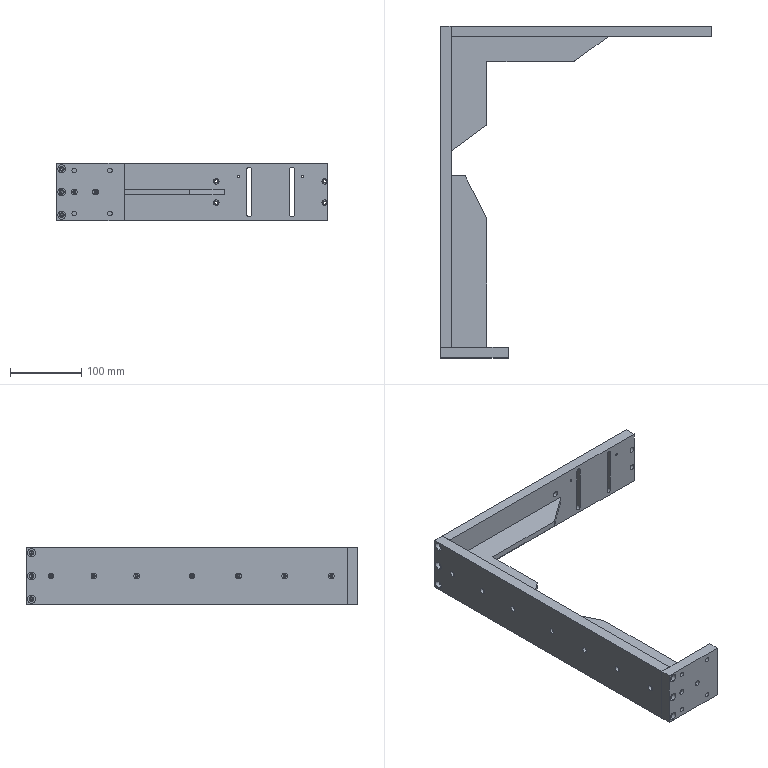Part | SolidWorks | 5 solids | 274 faces | box 380 x 465 x 80 mm | volume 1262568 mm3 | cylinder 162 | plane 70 | cone 42 | commonest cylinder face diameters 3.3 x34 4.5 x34 8 x26 6.6 x24 11 x24 5 x12